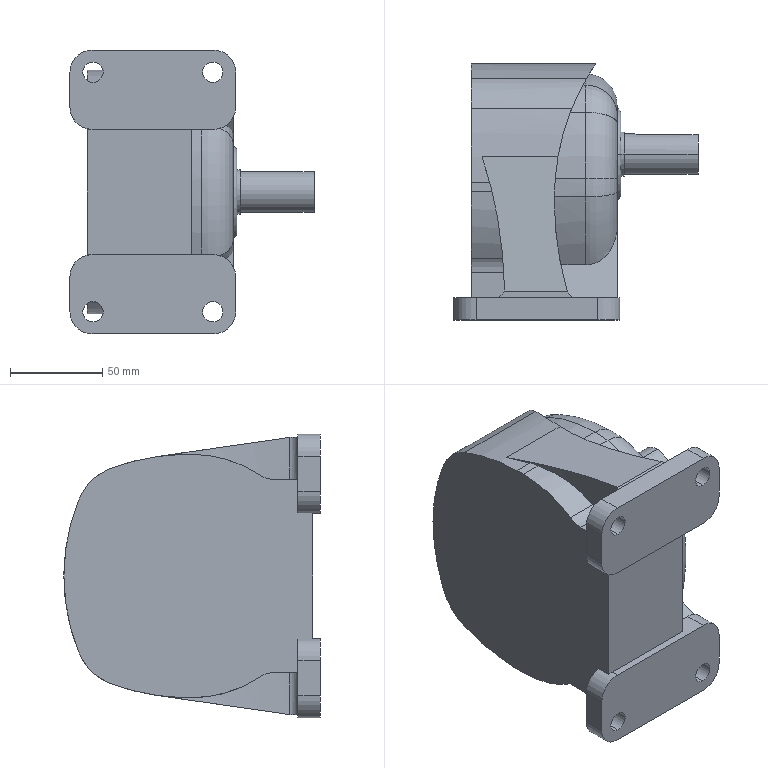Part | STEP file | G3L22N30-MM02TNNTNXH6-Part-4 | 1 solid | 115 faces | box 132.5 x 139 x 154 mm | volume 1248775 mm3 | cylinder 59 | plane 38 | torus 14 | cone 4 | commonest cylinder face diameters 24 x12 11 x8 10 x5 168 x4 250 x4 340 x4